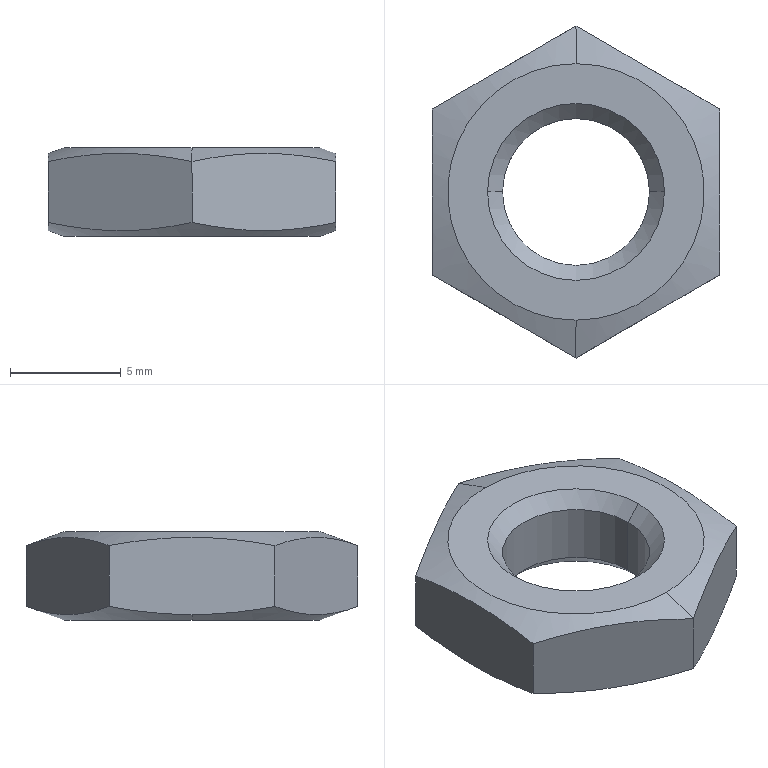Part | SolidWorks | features BaseBody 1 | 1 solid | 18 faces | box 13 x 15.011 x 4 mm | volume 419.435 mm3 | cone 8 | plane 8 | cylinder 2 | commonest cylinder face diameters 6.647 x2
STEP:
#1=CARTESIAN_POINT('',(5.8,0.,0.));
#2=VERTEX_POINT('',#1);
#3=CARTESIAN_POINT('',(-5.8,0.,0.));
#4=VERTEX_POINT('',#3);
#5=CARTESIAN_POINT('',(0.,0.,0.));
#6=DIRECTION('',(0.,0.,1.));
#7=DIRECTION('',(1.,0.,0.));
#8=AXIS2_PLACEMENT_3D('',#5,#6,#7);
#9=CIRCLE('',#8,5.8);
#10=EDGE_CURVE('',#2,#4,#9,.T.);
#11=ORIENTED_EDGE('',*,*,#10,.T.);
#12=CARTESIAN_POINT('',(-6.5,0.,0.2548));
#13=VERTEX_POINT('',#12);
#14=CARTESIAN_POINT('',(-7.516,0.,0.6245));
#15=DIRECTION('',(-0.9397,0.,0.342));
#16=VECTOR('',#15,1000.);
#17=LINE('',#14,#16);
#18=EDGE_CURVE('',#4,#13,#17,.T.);
#19=ORIENTED_EDGE('',*,*,#18,.T.);
#20=CARTESIAN_POINT('',(-6.5,3.753,0.6208));
#21=VERTEX_POINT('',#20);
#22=CARTESIAN_POINT('',(-6.5,0.,0.2548));
#23=CARTESIAN_POINT('',(-6.5,1.263,0.2548));
#24=CARTESIAN_POINT('',(-6.5,2.512,0.395));
#25=CARTESIAN_POINT('',(-6.5,3.753,0.6208));
#26=B_SPLINE_CURVE_WITH_KNOTS('',3,(#22,#23,#24,#25),.UNSPECIFIED.,.F.,.F.,(4,4),(0.,0.003771),.UNSPECIFIED.);
#27=EDGE_CURVE('',#13,#21,#26,.T.);
#28=ORIENTED_EDGE('',*,*,#27,.T.);
#29=CARTESIAN_POINT('',(-0.000000052,7.506,0.6208));
#30=VERTEX_POINT('',#29);
#31=CARTESIAN_POINT('',(-6.5,3.753,0.6208));
#32=CARTESIAN_POINT('',(-5.958,4.066,0.5069));
#33=CARTESIAN_POINT('',(-5.417,4.378,0.4145));
#34=CARTESIAN_POINT('',(-4.333,5.004,0.2882));
#35=CARTESIAN_POINT('',(-3.25,5.629,0.2213));
#36=CARTESIAN_POINT('',(-2.167,6.255,0.2882));
#37=CARTESIAN_POINT('',(-1.083,6.88,0.4145));
#38=CARTESIAN_POINT('',(-0.5417,7.193,0.5069));
#39=CARTESIAN_POINT('',(-0.000000052,7.506,0.6208));
#40=B_SPLINE_CURVE_WITH_KNOTS('',3,(#31,#32,#33,#34,#35,#36,#37,#38,#39),.UNSPECIFIED.,.F.,.F.,(4,2,1,2,4),(0.,0.001876,0.003753,0.005629,0.007506),.UNSPECIFIED.);
#41=EDGE_CURVE('',#21,#30,#40,.T.);
#42=ORIENTED_EDGE('',*,*,#41,.T.);
#43=CARTESIAN_POINT('',(6.5,3.753,0.6208));
#44=VERTEX_POINT('',#43);
#45=CARTESIAN_POINT('',(-0.000000052,7.506,0.6208));
#46=CARTESIAN_POINT('',(0.5417,7.193,0.5069));
#47=CARTESIAN_POINT('',(1.083,6.88,0.4145));
#48=CARTESIAN_POINT('',(2.167,6.255,0.2882));
#49=CARTESIAN_POINT('',(3.25,5.629,0.2213));
#50=CARTESIAN_POINT('',(4.333,5.004,0.2882));
#51=CARTESIAN_POINT('',(5.417,4.378,0.4145));
#52=CARTESIAN_POINT('',(5.958,4.066,0.5069));
#53=CARTESIAN_POINT('',(6.5,3.753,0.6208));
#54=B_SPLINE_CURVE_WITH_KNOTS('',3,(#45,#46,#47,#48,#49,#50,#51,#52,#53),.UNSPECIFIED.,.F.,.F.,(4,2,1,2,4),(0.,0.001876,0.003753,0.005629,0.007506),.UNSPECIFIED.);
#55=EDGE_CURVE('',#30,#44,#54,.T.);
#56=ORIENTED_EDGE('',*,*,#55,.T.);
#57=CARTESIAN_POINT('',(6.5,0.,0.2548));
#58=VERTEX_POINT('',#57);
#59=CARTESIAN_POINT('',(6.5,3.753,0.6208));
#60=CARTESIAN_POINT('',(6.5,2.512,0.395));
#61=CARTESIAN_POINT('',(6.5,1.263,0.2548));
#62=CARTESIAN_POINT('',(6.5,0.,0.2548));
#63=B_SPLINE_CURVE_WITH_KNOTS('',3,(#59,#60,#61,#62),.UNSPECIFIED.,.F.,.F.,(4,4),(0.,0.003771),.UNSPECIFIED.);
#64=EDGE_CURVE('',#44,#58,#63,.T.);
#65=ORIENTED_EDGE('',*,*,#64,.T.);
#66=CARTESIAN_POINT('',(7.516,0.,0.6245));
#67=DIRECTION('',(0.9397,0.,0.342));
#68=VECTOR('',#67,1000.);
#69=LINE('',#66,#68);
#70=EDGE_CURVE('',#2,#58,#69,.T.);
#71=ORIENTED_EDGE('',*,*,#70,.F.);
#72=EDGE_LOOP('',(#11,#19,#28,#42,#56,#65,#71));
#73=FACE_OUTER_BOUND('',#72,.T.);
#74=CARTESIAN_POINT('',(0.,0.,0.6245));
#75=DIRECTION('',(0.,0.,1.));
#76=DIRECTION('',(1.,0.,0.));
#77=AXIS2_PLACEMENT_3D('',#74,#75,#76);
#78=CONICAL_SURFACE('',#77,7.516,1.222);
#79=ADVANCED_FACE('',(#73),#78,.T.);
#80=CARTESIAN_POINT('',(3.324,0.,0.6765));
#81=VERTEX_POINT('',#80);
#82=CARTESIAN_POINT('',(-3.324,0.,0.6765));
#83=VERTEX_POINT('',#82);
#84=CARTESIAN_POINT('',(0.,0.,0.6765));
#85=DIRECTION('',(0.,0.,-1.));
#86=DIRECTION('',(-1.,0.,0.));
#87=AXIS2_PLACEMENT_3D('',#84,#85,#86);
#88=CIRCLE('',#87,3.324);
#89=EDGE_CURVE('',#81,#83,#88,.T.);
#90=ORIENTED_EDGE('',*,*,#89,.F.);
#91=CARTESIAN_POINT('',(4.,0.,0.));
#92=VERTEX_POINT('',#91);
#93=CARTESIAN_POINT('',(4.,0.,0.));
#94=DIRECTION('',(0.7071,0.,-0.7071));
#95=VECTOR('',#94,1000.);
#96=LINE('',#93,#95);
#97=EDGE_CURVE('',#81,#92,#96,.T.);
#98=ORIENTED_EDGE('',*,*,#97,.T.);
#99=CARTESIAN_POINT('',(-4.,0.,0.));
#100=VERTEX_POINT('',#99);
#101=CARTESIAN_POINT('',(0.,0.,0.));
#102=DIRECTION('',(0.,0.,-1.));
#103=DIRECTION('',(-1.,0.,0.));
#104=AXIS2_PLACEMENT_3D('',#101,#102,#103);
#105=CIRCLE('',#104,4.);
#106=EDGE_CURVE('',#92,#100,#105,.T.);
#107=ORIENTED_EDGE('',*,*,#106,.T.);
#108=CARTESIAN_POINT('',(-4.,0.,0.));
#109=DIRECTION('',(-0.7071,0.,-0.7071));
#110=VECTOR('',#109,1000.);
#111=LINE('',#108,#110);
#112=EDGE_CURVE('',#83,#100,#111,.T.);
#113=ORIENTED_EDGE('',*,*,#112,.F.);
#114=EDGE_LOOP('',(#90,#98,#107,#113));
#115=FACE_OUTER_BOUND('',#114,.T.);
#116=CARTESIAN_POINT('',(0.,0.,0.));
#117=DIRECTION('',(0.,0.,-1.));
#118=DIRECTION('',(-1.,0.,0.));
#119=AXIS2_PLACEMENT_3D('',#116,#117,#118);
#120=CONICAL_SURFACE('',#119,4.,0.7854);
#121=ADVANCED_FACE('',(#115),#120,.F.);
#122=ORIENTED_EDGE('',*,*,#89,.T.);
#123=CARTESIAN_POINT('',(-3.324,0.,3.324));
#124=VERTEX_POINT('',#123);
#125=CARTESIAN_POINT('',(-3.324,0.,0.));
#126=DIRECTION('',(0.,0.,1.));
#127=VECTOR('',#126,1000.);
#128=LINE('',#125,#127);
#129=EDGE_CURVE('',#83,#124,#128,.T.);
#130=ORIENTED_EDGE('',*,*,#129,.T.);
#131=CARTESIAN_POINT('',(3.324,0.,3.324));
#132=VERTEX_POINT('',#131);
#133=CARTESIAN_POINT('',(0.,0.,3.324));
#134=DIRECTION('',(0.,0.,-1.));
#135=DIRECTION('',(1.,0.,0.));
#136=AXIS2_PLACEMENT_3D('',#133,#134,#135);
#137=CIRCLE('',#136,3.324);
#138=EDGE_CURVE('',#132,#124,#137,.T.);
#139=ORIENTED_EDGE('',*,*,#138,.F.);
#140=CARTESIAN_POINT('',(3.324,0.,0.));
#141=DIRECTION('',(0.,0.,1.));
#142=VECTOR('',#141,1000.);
#143=LINE('',#140,#142);
#144=EDGE_CURVE('',#81,#132,#143,.T.);
#145=ORIENTED_EDGE('',*,*,#144,.F.);
#146=EDGE_LOOP('',(#122,#130,#139,#145));
#147=FACE_OUTER_BOUND('',#146,.T.);
#148=CARTESIAN_POINT('',(0.,0.,0.));
#149=DIRECTION('',(0.,0.,1.));
#150=DIRECTION('',(1.,0.,0.));
#151=AXIS2_PLACEMENT_3D('',#148,#149,#150);
#152=CYLINDRICAL_SURFACE('',#151,3.324);
#153=ADVANCED_FACE('',(#147),#152,.F.);
#154=CARTESIAN_POINT('',(0.,5.8,4.));
#155=VERTEX_POINT('',#154);
#156=CARTESIAN_POINT('',(0.,-5.8,4.));
#157=VERTEX_POINT('',#156);
#158=CARTESIAN_POINT('',(0.,0.,4.));
#159=DIRECTION('',(0.,0.,-1.));
#160=DIRECTION('',(0.,1.,0.));
#161=AXIS2_PLACEMENT_3D('',#158,#159,#160);
#162=CIRCLE('',#161,5.8);
#163=EDGE_CURVE('',#155,#157,#162,.T.);
#164=ORIENTED_EDGE('',*,*,#163,.T.);
#165=CARTESIAN_POINT('',(-0.000000014,-7.506,3.379));
#166=VERTEX_POINT('',#165);
#167=CARTESIAN_POINT('',(0.,-7.516,3.376));
#168=DIRECTION('',(0.,-0.9397,-0.342));
#169=VECTOR('',#168,1000.);
#170=LINE('',#167,#169);
#171=EDGE_CURVE('',#157,#166,#170,.T.);
#172=ORIENTED_EDGE('',*,*,#171,.T.);
#173=CARTESIAN_POINT('',(6.5,-3.753,3.379));
#174=VERTEX_POINT('',#173);
#175=CARTESIAN_POINT('',(-0.000000014,-7.506,3.379));
#176=CARTESIAN_POINT('',(0.5417,-7.193,3.493));
#177=CARTESIAN_POINT('',(1.083,-6.88,3.585));
#178=CARTESIAN_POINT('',(2.167,-6.255,3.712));
#179=CARTESIAN_POINT('',(3.25,-5.629,3.779));
#180=CARTESIAN_POINT('',(4.333,-5.004,3.712));
#181=CARTESIAN_POINT('',(5.417,-4.378,3.585));
#182=CARTESIAN_POINT('',(5.958,-4.066,3.493));
#183=CARTESIAN_POINT('',(6.5,-3.753,3.379));
#184=B_SPLINE_CURVE_WITH_KNOTS('',3,(#175,#176,#177,#178,#179,#180,#181,#182,#183),.UNSPECIFIED.,.F.,.F.,(4,2,1,2,4),(0.,0.001876,0.003753,0.005629,0.007506),.UNSPECIFIED.);
#185=EDGE_CURVE('',#166,#174,#184,.T.);
#186=ORIENTED_EDGE('',*,*,#185,.T.);
#187=CARTESIAN_POINT('',(6.5,3.753,3.379));
#188=VERTEX_POINT('',#187);
#189=CARTESIAN_POINT('',(6.5,-3.753,3.379));
#190=CARTESIAN_POINT('',(6.5,-3.127,3.493));
#191=CARTESIAN_POINT('',(6.5,-2.502,3.585));
#192=CARTESIAN_POINT('',(6.5,-1.251,3.712));
#193=CARTESIAN_POINT('',(6.5,0.000000004,3.779));
#194=CARTESIAN_POINT('',(6.5,1.251,3.712));
#195=CARTESIAN_POINT('',(6.5,2.502,3.585));
#196=CARTESIAN_POINT('',(6.5,3.127,3.493));
#197=CARTESIAN_POINT('',(6.5,3.753,3.379));
#198=B_SPLINE_CURVE_WITH_KNOTS('',3,(#189,#190,#191,#192,#193,#194,#195,#196,#197),.UNSPECIFIED.,.F.,.F.,(4,2,1,2,4),(0.,0.001876,0.003753,0.005629,0.007506),.UNSPECIFIED.);
#199=EDGE_CURVE('',#174,#188,#198,.T.);
#200=ORIENTED_EDGE('',*,*,#199,.T.);
#201=CARTESIAN_POINT('',(-0.000000003,7.506,3.379));
#202=VERTEX_POINT('',#201);
#203=CARTESIAN_POINT('',(6.5,3.753,3.379));
#204=CARTESIAN_POINT('',(5.958,4.066,3.493));
#205=CARTESIAN_POINT('',(5.417,4.378,3.585));
#206=CARTESIAN_POINT('',(4.333,5.004,3.712));
#207=CARTESIAN_POINT('',(3.25,5.629,3.779));
#208=CARTESIAN_POINT('',(2.167,6.255,3.712));
#209=CARTESIAN_POINT('',(1.083,6.88,3.585));
#210=CARTESIAN_POINT('',(0.5417,7.193,3.493));
#211=CARTESIAN_POINT('',(-0.000000003,7.506,3.379));
#212=B_SPLINE_CURVE_WITH_KNOTS('',3,(#203,#204,#205,#206,#207,#208,#209,#210,#211),.UNSPECIFIED.,.F.,.F.,(4,2,1,2,4),(0.,0.001876,0.003753,0.005629,0.007506),.UNSPECIFIED.);
#213=EDGE_CURVE('',#188,#202,#212,.T.);
#214=ORIENTED_EDGE('',*,*,#213,.T.);
#215=CARTESIAN_POINT('',(0.,7.516,3.376));
#216=DIRECTION('',(0.,0.9397,-0.342));
#217=VECTOR('',#216,1000.);
#218=LINE('',#215,#217);
#219=EDGE_CURVE('',#155,#202,#218,.T.);
#220=ORIENTED_EDGE('',*,*,#219,.F.);
#221=EDGE_LOOP('',(#164,#172,#186,#200,#214,#220));
#222=FACE_OUTER_BOUND('',#221,.T.);
#223=CARTESIAN_POINT('',(0.,0.,3.376));
#224=DIRECTION('',(0.,0.,-1.));
#225=DIRECTION('',(0.,1.,0.));
#226=AXIS2_PLACEMENT_3D('',#223,#224,#225);
#227=CONICAL_SURFACE('',#226,7.516,1.222);
#228=ADVANCED_FACE('',(#222),#227,.T.);
#229=ORIENTED_EDGE('',*,*,#138,.T.);
#230=CARTESIAN_POINT('',(-4.,0.,4.));
#231=VERTEX_POINT('',#230);
#232=CARTESIAN_POINT('',(-4.,0.,4.));
#233=DIRECTION('',(-0.7071,0.,0.7071));
#234=VECTOR('',#233,1000.);
#235=LINE('',#232,#234);
#236=EDGE_CURVE('',#124,#231,#235,.T.);
#237=ORIENTED_EDGE('',*,*,#236,.T.);
#238=CARTESIAN_POINT('',(4.,0.,4.));
#239=VERTEX_POINT('',#238);
#240=CARTESIAN_POINT('',(0.,0.,4.));
#241=DIRECTION('',(0.,0.,-1.));
#242=DIRECTION('',(1.,0.,0.));
#243=AXIS2_PLACEMENT_3D('',#240,#241,#242);
#244=CIRCLE('',#243,4.);
#245=EDGE_CURVE('',#239,#231,#244,.T.);
#246=ORIENTED_EDGE('',*,*,#245,.F.);
#247=CARTESIAN_POINT('',(4.,0.,4.));
#248=DIRECTION('',(0.7071,0.,0.7071));
#249=VECTOR('',#248,1000.);
#250=LINE('',#247,#249);
#251=EDGE_CURVE('',#132,#239,#250,.T.);
#252=ORIENTED_EDGE('',*,*,#251,.F.);
#253=EDGE_LOOP('',(#229,#237,#246,#252));
#254=FACE_OUTER_BOUND('',#253,.T.);
#255=CARTESIAN_POINT('',(0.,0.,4.));
#256=DIRECTION('',(0.,0.,1.));
#257=DIRECTION('',(1.,0.,0.));
#258=AXIS2_PLACEMENT_3D('',#255,#256,#257);
#259=CONICAL_SURFACE('',#258,4.,0.7854);
#260=ADVANCED_FACE('',(#254),#259,.F.);
#261=ORIENTED_EDGE('',*,*,#10,.F.);
#262=CARTESIAN_POINT('',(0.,0.,0.));
#263=DIRECTION('',(0.,0.,1.));
#264=DIRECTION('',(1.,0.,0.));
#265=AXIS2_PLACEMENT_3D('',#262,#263,#264);
#266=CIRCLE('',#265,5.8);
#267=EDGE_CURVE('',#4,#2,#266,.T.);
#268=ORIENTED_EDGE('',*,*,#267,.F.);
#269=EDGE_LOOP('',(#261,#268));
#270=FACE_OUTER_BOUND('',#269,.T.);
#271=CARTESIAN_POINT('',(0.,0.,0.));
#272=DIRECTION('',(0.,0.,-1.));
#273=DIRECTION('',(-1.,0.,0.));
#274=AXIS2_PLACEMENT_3D('',#271,#272,#273);
#275=CIRCLE('',#274,4.);
#276=EDGE_CURVE('',#100,#92,#275,.T.);
#277=ORIENTED_EDGE('',*,*,#276,.F.);
#278=ORIENTED_EDGE('',*,*,#106,.F.);
#279=EDGE_LOOP('',(#277,#278));
#280=FACE_BOUND('',#279,.T.);
#281=CARTESIAN_POINT('',(0.,0.,0.));
#282=DIRECTION('',(0.,0.,1.));
#283=DIRECTION('',(1.,0.,0.));
#284=AXIS2_PLACEMENT_3D('',#281,#282,#283);
#285=PLANE('',#284);
#286=ADVANCED_FACE('',(#270,#280),#285,.F.);
#287=ORIENTED_EDGE('',*,*,#18,.F.);
#288=ORIENTED_EDGE('',*,*,#267,.T.);
#289=ORIENTED_EDGE('',*,*,#70,.T.);
#290=CARTESIAN_POINT('',(6.5,-3.753,0.6208));
#291=VERTEX_POINT('',#290);
#292=CARTESIAN_POINT('',(6.5,0.,0.2548));
#293=CARTESIAN_POINT('',(6.5,-1.263,0.2548));
#294=CARTESIAN_POINT('',(6.5,-2.512,0.395));
#295=CARTESIAN_POINT('',(6.5,-3.753,0.6208));
#296=B_SPLINE_CURVE_WITH_KNOTS('',3,(#292,#293,#294,#295),.UNSPECIFIED.,.F.,.F.,(4,4),(0.003771,0.007541),.UNSPECIFIED.);
#297=EDGE_CURVE('',#58,#291,#296,.T.);
#298=ORIENTED_EDGE('',*,*,#297,.T.);
#299=CARTESIAN_POINT('',(0.000000044,-7.506,0.6208));
#300=VERTEX_POINT('',#299);
#301=CARTESIAN_POINT('',(6.5,-3.753,0.6208));
#302=CARTESIAN_POINT('',(5.958,-4.066,0.5069));
#303=CARTESIAN_POINT('',(5.417,-4.378,0.4145));
#304=CARTESIAN_POINT('',(4.333,-5.004,0.2882));
#305=CARTESIAN_POINT('',(3.25,-5.629,0.2213));
#306=CARTESIAN_POINT('',(2.167,-6.255,0.2882));
#307=CARTESIAN_POINT('',(1.083,-6.88,0.4145));
#308=CARTESIAN_POINT('',(0.5417,-7.193,0.5069));
#309=CARTESIAN_POINT('',(0.000000044,-7.506,0.6208));
#310=B_SPLINE_CURVE_WITH_KNOTS('',3,(#301,#302,#303,#304,#305,#306,#307,#308,#309),.UNSPECIFIED.,.F.,.F.,(4,2,1,2,4),(0.,0.001876,0.003753,0.005629,0.007506),.UNSPECIFIED.);
#311=EDGE_CURVE('',#291,#300,#310,.T.);
#312=ORIENTED_EDGE('',*,*,#311,.T.);
#313=CARTESIAN_POINT('',(-6.5,-3.753,0.6208));
#314=VERTEX_POINT('',#313);
#315=CARTESIAN_POINT('',(0.000000044,-7.506,0.6208));
#316=CARTESIAN_POINT('',(-0.5417,-7.193,0.5069));
#317=CARTESIAN_POINT('',(-1.083,-6.88,0.4145));
#318=CARTESIAN_POINT('',(-2.167,-6.255,0.2882));
#319=CARTESIAN_POINT('',(-3.25,-5.629,0.2213));
#320=CARTESIAN_POINT('',(-4.333,-5.004,0.2882));
#321=CARTESIAN_POINT('',(-5.417,-4.378,0.4145));
#322=CARTESIAN_POINT('',(-5.958,-4.066,0.5069));
#323=CARTESIAN_POINT('',(-6.5,-3.753,0.6208));
#324=B_SPLINE_CURVE_WITH_KNOTS('',3,(#315,#316,#317,#318,#319,#320,#321,#322,#323),.UNSPECIFIED.,.F.,.F.,(4,2,1,2,4),(0.,0.001876,0.003753,0.005629,0.007506),.UNSPECIFIED.);
#325=EDGE_CURVE('',#300,#314,#324,.T.);
#326=ORIENTED_EDGE('',*,*,#325,.T.);
#327=CARTESIAN_POINT('',(-6.5,-3.753,0.6208));
#328=CARTESIAN_POINT('',(-6.5,-2.512,0.395));
#329=CARTESIAN_POINT('',(-6.5,-1.263,0.2548));
#330=CARTESIAN_POINT('',(-6.5,0.,0.2548));
#331=B_SPLINE_CURVE_WITH_KNOTS('',3,(#327,#328,#329,#330),.UNSPECIFIED.,.F.,.F.,(4,4),(-0.003771,0.),.UNSPECIFIED.);
#332=EDGE_CURVE('',#314,#13,#331,.T.);
#333=ORIENTED_EDGE('',*,*,#332,.T.);
#334=EDGE_LOOP('',(#287,#288,#289,#298,#312,#326,#333));
#335=FACE_OUTER_BOUND('',#334,.T.);
#336=CARTESIAN_POINT('',(0.,0.,0.6245));
#337=DIRECTION('',(0.,0.,1.));
#338=DIRECTION('',(1.,0.,0.));
#339=AXIS2_PLACEMENT_3D('',#336,#337,#338);
#340=CONICAL_SURFACE('',#339,7.516,1.222);
#341=ADVANCED_FACE('',(#335),#340,.T.);
#342=ORIENTED_EDGE('',*,*,#97,.F.);
#343=CARTESIAN_POINT('',(0.,0.,0.6765));
#344=DIRECTION('',(0.,0.,-1.));
#345=DIRECTION('',(-1.,0.,0.));
#346=AXIS2_PLACEMENT_3D('',#343,#344,#345);
#347=CIRCLE('',#346,3.324);
#348=EDGE_CURVE('',#83,#81,#347,.T.);
#349=ORIENTED_EDGE('',*,*,#348,.F.);
#350=ORIENTED_EDGE('',*,*,#112,.T.);
#351=ORIENTED_EDGE('',*,*,#276,.T.);
#352=EDGE_LOOP('',(#342,#349,#350,#351));
#353=FACE_OUTER_BOUND('',#352,.T.);
#354=CARTESIAN_POINT('',(0.,0.,0.));
#355=DIRECTION('',(0.,0.,-1.));
#356=DIRECTION('',(-1.,0.,0.));
#357=AXIS2_PLACEMENT_3D('',#354,#355,#356);
#358=CONICAL_SURFACE('',#357,4.,0.7854);
#359=ADVANCED_FACE('',(#353),#358,.F.);
#360=CARTESIAN_POINT('',(6.5,-3.753,4.));
#361=DIRECTION('',(0.,0.,1.));
#362=VECTOR('',#361,1000.);
#363=LINE('',#360,#362);
#364=EDGE_CURVE('',#291,#174,#363,.T.);
#365=ORIENTED_EDGE('',*,*,#364,.F.);
#366=ORIENTED_EDGE('',*,*,#297,.F.);
#367=ORIENTED_EDGE('',*,*,#64,.F.);
#368=CARTESIAN_POINT('',(6.5,3.753,4.));
#369=DIRECTION('',(0.,0.,-1.));
#370=VECTOR('',#369,1000.);
#371=LINE('',#368,#370);
#372=EDGE_CURVE('',#188,#44,#371,.T.);
#373=ORIENTED_EDGE('',*,*,#372,.F.);
#374=ORIENTED_EDGE('',*,*,#199,.F.);
#375=EDGE_LOOP('',(#365,#366,#367,#373,#374));
#376=FACE_OUTER_BOUND('',#375,.T.);
#377=CARTESIAN_POINT('',(6.5,-3.753,4.));
#378=DIRECTION('',(-1.,0.,0.));
#379=DIRECTION('',(0.,0.,1.));
#380=AXIS2_PLACEMENT_3D('',#377,#378,#379);
#381=PLANE('',#380);
#382=ADVANCED_FACE('',(#376),#381,.F.);
#383=ORIENTED_EDGE('',*,*,#372,.T.);
#384=ORIENTED_EDGE('',*,*,#55,.F.);
#385=CARTESIAN_POINT('',(-0.000000006,7.506,4.));
#386=DIRECTION('',(0.,0.,-1.));
#387=VECTOR('',#386,1000.);
#388=LINE('',#385,#387);
#389=EDGE_CURVE('',#202,#30,#388,.T.);
#390=ORIENTED_EDGE('',*,*,#389,.F.);
#391=ORIENTED_EDGE('',*,*,#213,.F.);
#392=EDGE_LOOP('',(#383,#384,#390,#391));
#393=FACE_OUTER_BOUND('',#392,.T.);
#394=CARTESIAN_POINT('',(6.5,3.753,4.));
#395=DIRECTION('',(-0.5,-0.866,0.));
#396=DIRECTION('',(0.866,-0.5,0.));
#397=AXIS2_PLACEMENT_3D('',#394,#395,#396);
#398=PLANE('',#397);
#399=ADVANCED_FACE('',(#393),#398,.F.);
#400=ORIENTED_EDGE('',*,*,#389,.T.);
#401=ORIENTED_EDGE('',*,*,#41,.F.);
#402=CARTESIAN_POINT('',(-6.5,3.753,3.379));
#403=VERTEX_POINT('',#402);
#404=CARTESIAN_POINT('',(-6.5,3.753,4.));
#405=DIRECTION('',(0.,0.,-1.));
#406=VECTOR('',#405,1000.);
#407=LINE('',#404,#406);
#408=EDGE_CURVE('',#403,#21,#407,.T.);
#409=ORIENTED_EDGE('',*,*,#408,.F.);
#410=CARTESIAN_POINT('',(-0.000000003,7.506,3.379));
#411=CARTESIAN_POINT('',(-0.5417,7.193,3.493));
#412=CARTESIAN_POINT('',(-1.083,6.88,3.585));
#413=CARTESIAN_POINT('',(-2.167,6.255,3.712));
#414=CARTESIAN_POINT('',(-3.25,5.629,3.779));
#415=CARTESIAN_POINT('',(-4.333,5.004,3.712));
#416=CARTESIAN_POINT('',(-5.417,4.378,3.585));
#417=CARTESIAN_POINT('',(-5.958,4.066,3.493));
#418=CARTESIAN_POINT('',(-6.5,3.753,3.379));
#419=B_SPLINE_CURVE_WITH_KNOTS('',3,(#410,#411,#412,#413,#414,#415,#416,#417,#418),.UNSPECIFIED.,.F.,.F.,(4,2,1,2,4),(0.,0.001876,0.003753,0.005629,0.007506),.UNSPECIFIED.);
#420=EDGE_CURVE('',#202,#403,#419,.T.);
#421=ORIENTED_EDGE('',*,*,#420,.F.);
#422=EDGE_LOOP('',(#400,#401,#409,#421));
#423=FACE_OUTER_BOUND('',#422,.T.);
#424=CARTESIAN_POINT('',(0.,7.506,4.));
#425=DIRECTION('',(0.5,-0.866,0.));
#426=DIRECTION('',(0.866,0.5,0.));
#427=AXIS2_PLACEMENT_3D('',#424,#425,#426);
#428=PLANE('',#427);
#429=ADVANCED_FACE('',(#423),#428,.F.);
#430=ORIENTED_EDGE('',*,*,#408,.T.);
#431=ORIENTED_EDGE('',*,*,#27,.F.);
#432=ORIENTED_EDGE('',*,*,#332,.F.);
#433=CARTESIAN_POINT('',(-6.5,-3.753,3.379));
#434=VERTEX_POINT('',#433);
#435=CARTESIAN_POINT('',(-6.5,-3.753,4.));
#436=DIRECTION('',(0.,0.,-1.));
#437=VECTOR('',#436,1000.);
#438=LINE('',#435,#437);
#439=EDGE_CURVE('',#434,#314,#438,.T.);
#440=ORIENTED_EDGE('',*,*,#439,.F.);
#441=CARTESIAN_POINT('',(-6.5,3.753,3.379));
#442=CARTESIAN_POINT('',(-6.5,3.127,3.493));
#443=CARTESIAN_POINT('',(-6.5,2.502,3.585));
#444=CARTESIAN_POINT('',(-6.5,1.251,3.712));
#445=CARTESIAN_POINT('',(-6.5,0.000000009,3.779));
#446=CARTESIAN_POINT('',(-6.5,-1.251,3.712));
#447=CARTESIAN_POINT('',(-6.5,-2.502,3.585));
#448=CARTESIAN_POINT('',(-6.5,-3.127,3.493));
#449=CARTESIAN_POINT('',(-6.5,-3.753,3.379));
#450=B_SPLINE_CURVE_WITH_KNOTS('',3,(#441,#442,#443,#444,#445,#446,#447,#448,#449),.UNSPECIFIED.,.F.,.F.,(4,2,1,2,4),(0.,0.001876,0.003753,0.005629,0.007506),.UNSPECIFIED.);
#451=EDGE_CURVE('',#403,#434,#450,.T.);
#452=ORIENTED_EDGE('',*,*,#451,.F.);
#453=EDGE_LOOP('',(#430,#431,#432,#440,#452));
#454=FACE_OUTER_BOUND('',#453,.T.);
#455=CARTESIAN_POINT('',(-6.5,3.753,4.));
#456=DIRECTION('',(1.,0.,0.));
#457=DIRECTION('',(0.,0.,-1.));
#458=AXIS2_PLACEMENT_3D('',#455,#456,#457);
#459=PLANE('',#458);
#460=ADVANCED_FACE('',(#454),#459,.F.);
#461=ORIENTED_EDGE('',*,*,#439,.T.);
#462=ORIENTED_EDGE('',*,*,#325,.F.);
#463=CARTESIAN_POINT('',(-0.000000009,-7.506,4.));
#464=DIRECTION('',(0.,0.,-1.));
#465=VECTOR('',#464,1000.);
#466=LINE('',#463,#465);
#467=EDGE_CURVE('',#166,#300,#466,.T.);
#468=ORIENTED_EDGE('',*,*,#467,.F.);
#469=CARTESIAN_POINT('',(-6.5,-3.753,3.379));
#470=CARTESIAN_POINT('',(-5.958,-4.066,3.493));
#471=CARTESIAN_POINT('',(-5.417,-4.378,3.585));
#472=CARTESIAN_POINT('',(-4.333,-5.004,3.712));
#473=CARTESIAN_POINT('',(-3.25,-5.629,3.779));
#474=CARTESIAN_POINT('',(-2.167,-6.255,3.712));
#475=CARTESIAN_POINT('',(-1.083,-6.88,3.585));
#476=CARTESIAN_POINT('',(-0.5417,-7.193,3.493));
#477=CARTESIAN_POINT('',(-0.000000014,-7.506,3.379));
#478=B_SPLINE_CURVE_WITH_KNOTS('',3,(#469,#470,#471,#472,#473,#474,#475,#476,#477),.UNSPECIFIED.,.F.,.F.,(4,2,1,2,4),(0.,0.001876,0.003753,0.005629,0.007506),.UNSPECIFIED.);
#479=EDGE_CURVE('',#434,#166,#478,.T.);
#480=ORIENTED_EDGE('',*,*,#479,.F.);
#481=EDGE_LOOP('',(#461,#462,#468,#480));
#482=FACE_OUTER_BOUND('',#481,.T.);
#483=CARTESIAN_POINT('',(-6.5,-3.753,4.));
#484=DIRECTION('',(0.5,0.866,0.));
#485=DIRECTION('',(-0.866,0.5,0.));
#486=AXIS2_PLACEMENT_3D('',#483,#484,#485);
#487=PLANE('',#486);
#488=ADVANCED_FACE('',(#482),#487,.F.);
#489=ORIENTED_EDGE('',*,*,#467,.T.);
#490=ORIENTED_EDGE('',*,*,#311,.F.);
#491=ORIENTED_EDGE('',*,*,#364,.T.);
#492=ORIENTED_EDGE('',*,*,#185,.F.);
#493=EDGE_LOOP('',(#489,#490,#491,#492));
#494=FACE_OUTER_BOUND('',#493,.T.);
#495=CARTESIAN_POINT('',(0.,-7.506,4.));
#496=DIRECTION('',(-0.5,0.866,0.));
#497=DIRECTION('',(-0.866,-0.5,0.));
#498=AXIS2_PLACEMENT_3D('',#495,#496,#497);
#499=PLANE('',#498);
#500=ADVANCED_FACE('',(#494),#499,.F.);
#501=ORIENTED_EDGE('',*,*,#129,.F.);
#502=ORIENTED_EDGE('',*,*,#348,.T.);
#503=ORIENTED_EDGE('',*,*,#144,.T.);
#504=CARTESIAN_POINT('',(0.,0.,3.324));
#505=DIRECTION('',(0.,0.,-1.));
#506=DIRECTION('',(1.,0.,0.));
#507=AXIS2_PLACEMENT_3D('',#504,#505,#506);
#508=CIRCLE('',#507,3.324);
#509=EDGE_CURVE('',#124,#132,#508,.T.);
#510=ORIENTED_EDGE('',*,*,#509,.F.);
#511=EDGE_LOOP('',(#501,#502,#503,#510));
#512=FACE_OUTER_BOUND('',#511,.T.);
#513=CARTESIAN_POINT('',(0.,0.,0.));
#514=DIRECTION('',(0.,0.,1.));
#515=DIRECTION('',(1.,0.,0.));
#516=AXIS2_PLACEMENT_3D('',#513,#514,#515);
#517=CYLINDRICAL_SURFACE('',#516,3.324);
#518=ADVANCED_FACE('',(#512),#517,.F.);
#519=ORIENTED_EDGE('',*,*,#171,.F.);
#520=CARTESIAN_POINT('',(0.,0.,4.));
#521=DIRECTION('',(0.,0.,-1.));
#522=DIRECTION('',(0.,1.,0.));
#523=AXIS2_PLACEMENT_3D('',#520,#521,#522);
#524=CIRCLE('',#523,5.8);
#525=EDGE_CURVE('',#157,#155,#524,.T.);
#526=ORIENTED_EDGE('',*,*,#525,.T.);
#527=ORIENTED_EDGE('',*,*,#219,.T.);
#528=ORIENTED_EDGE('',*,*,#420,.T.);
#529=ORIENTED_EDGE('',*,*,#451,.T.);
#530=ORIENTED_EDGE('',*,*,#479,.T.);
#531=EDGE_LOOP('',(#519,#526,#527,#528,#529,#530));
#532=FACE_OUTER_BOUND('',#531,.T.);
#533=CARTESIAN_POINT('',(0.,0.,3.376));
#534=DIRECTION('',(0.,0.,-1.));
#535=DIRECTION('',(0.,1.,0.));
#536=AXIS2_PLACEMENT_3D('',#533,#534,#535);
#537=CONICAL_SURFACE('',#536,7.516,1.222);
#538=ADVANCED_FACE('',(#532),#537,.T.);
#539=ORIENTED_EDGE('',*,*,#236,.F.);
#540=ORIENTED_EDGE('',*,*,#509,.T.);
#541=ORIENTED_EDGE('',*,*,#251,.T.);
#542=CARTESIAN_POINT('',(0.,0.,4.));
#543=DIRECTION('',(0.,0.,-1.));
#544=DIRECTION('',(1.,0.,0.));
#545=AXIS2_PLACEMENT_3D('',#542,#543,#544);
#546=CIRCLE('',#545,4.);
#547=EDGE_CURVE('',#231,#239,#546,.T.);
#548=ORIENTED_EDGE('',*,*,#547,.F.);
#549=EDGE_LOOP('',(#539,#540,#541,#548));
#550=FACE_OUTER_BOUND('',#549,.T.);
#551=CARTESIAN_POINT('',(0.,0.,4.));
#552=DIRECTION('',(0.,0.,1.));
#553=DIRECTION('',(1.,0.,0.));
#554=AXIS2_PLACEMENT_3D('',#551,#552,#553);
#555=CONICAL_SURFACE('',#554,4.,0.7854);
#556=ADVANCED_FACE('',(#550),#555,.F.);
#557=ORIENTED_EDGE('',*,*,#163,.F.);
#558=ORIENTED_EDGE('',*,*,#525,.F.);
#559=EDGE_LOOP('',(#557,#558));
#560=FACE_OUTER_BOUND('',#559,.T.);
#561=ORIENTED_EDGE('',*,*,#245,.T.);
#562=ORIENTED_EDGE('',*,*,#547,.T.);
#563=EDGE_LOOP('',(#561,#562));
#564=FACE_BOUND('',#563,.T.);
#565=CARTESIAN_POINT('',(0.,0.,4.));
#566=DIRECTION('',(0.,0.,1.));
#567=DIRECTION('',(1.,0.,0.));
#568=AXIS2_PLACEMENT_3D('',#565,#566,#567);
#569=PLANE('',#568);
#570=ADVANCED_FACE('',(#560,#564),#569,.T.);
#571=CLOSED_SHELL('',(#79,#121,#153,#228,#260,#286,#341,#359,#382,#399,#429,#460,#488,#500,#518,#538,#556,#570));
#572=MANIFOLD_SOLID_BREP('',#571);
#573=CARTESIAN_POINT('',(0.,0.,0.));
#574=DIRECTION('',(0.,0.,1.));
#575=DIRECTION('',(1.,0.,0.));
#576=AXIS2_PLACEMENT_3D('',#573,#574,#575);
#577=(LENGTH_UNIT()NAMED_UNIT(*)SI_UNIT(.MILLI.,.METRE.));
#578=UNCERTAINTY_MEASURE_WITH_UNIT(LENGTH_MEASURE(0.00001),#577,'','');
#579=(NAMED_UNIT(*)PLANE_ANGLE_UNIT()SI_UNIT($,.RADIAN.));
#580=(NAMED_UNIT(*)SI_UNIT($,.STERADIAN.)SOLID_ANGLE_UNIT());
#581=(GEOMETRIC_REPRESENTATION_CONTEXT(3)GLOBAL_UNCERTAINTY_ASSIGNED_CONTEXT((#578))GLOBAL_UNIT_ASSIGNED_CONTEXT((#577,#579,#580))REPRESENTATION_CONTEXT('',''));
#582=ADVANCED_BREP_SHAPE_REPRESENTATION('',(#572,#576),#581);